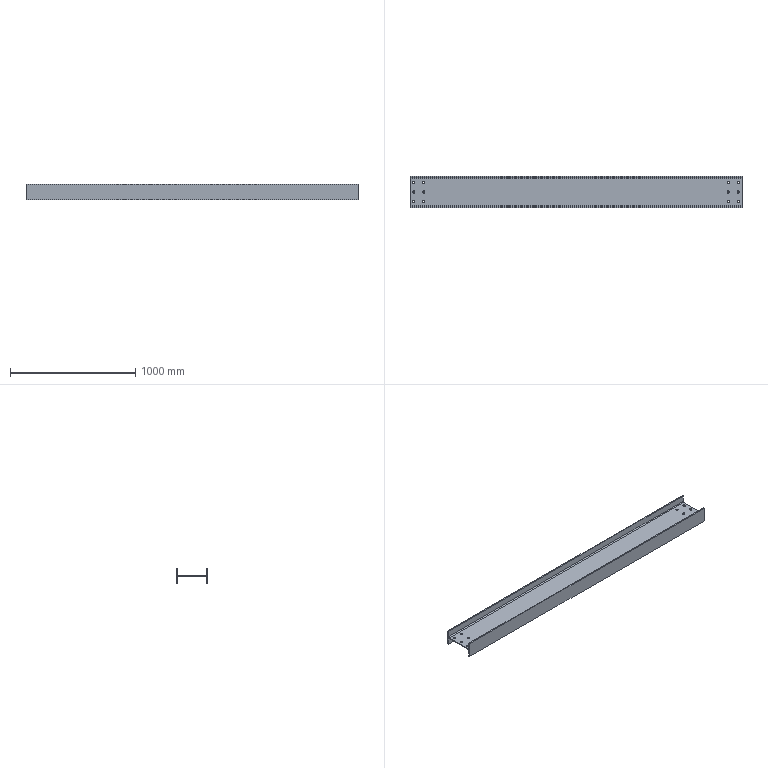Part | STEP file | 粉仓主梁9主体_Default<As Machined> | 1 solid | 42 faces | box 2655 x 250 x 125 mm | volume 9794957 mm3 | cylinder 28 | plane 14 | commonest cylinder face diameters 19 x24 16 x4